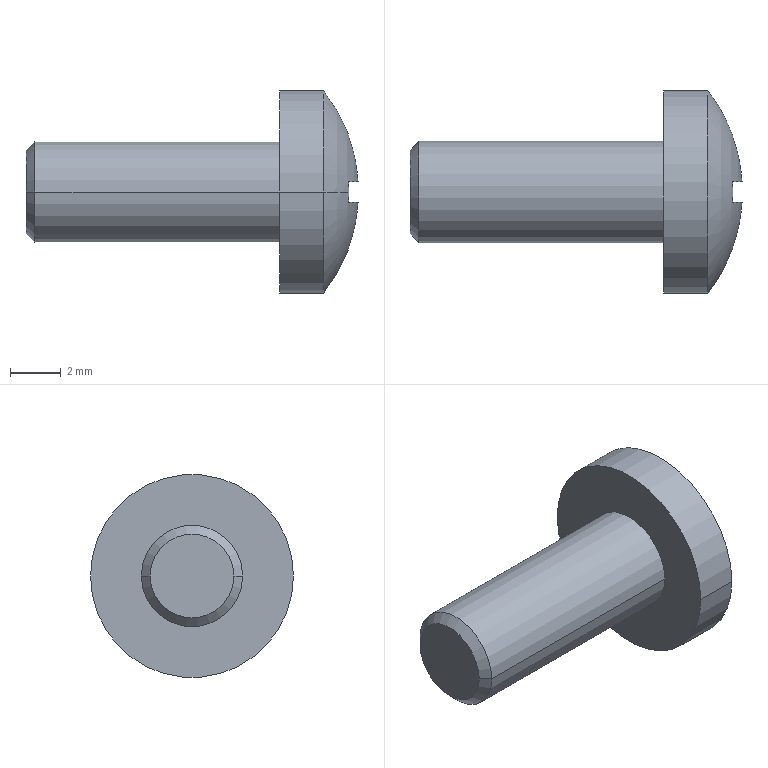Part | STEP file | SOLID | 1 solid | 23 faces | box 13.088 x 8 x 8 mm | volume 243.354 mm3 | plane 15 | cylinder 4 | sphere 2 | cone 2 | commonest cylinder face diameters 4 x2 8 x2